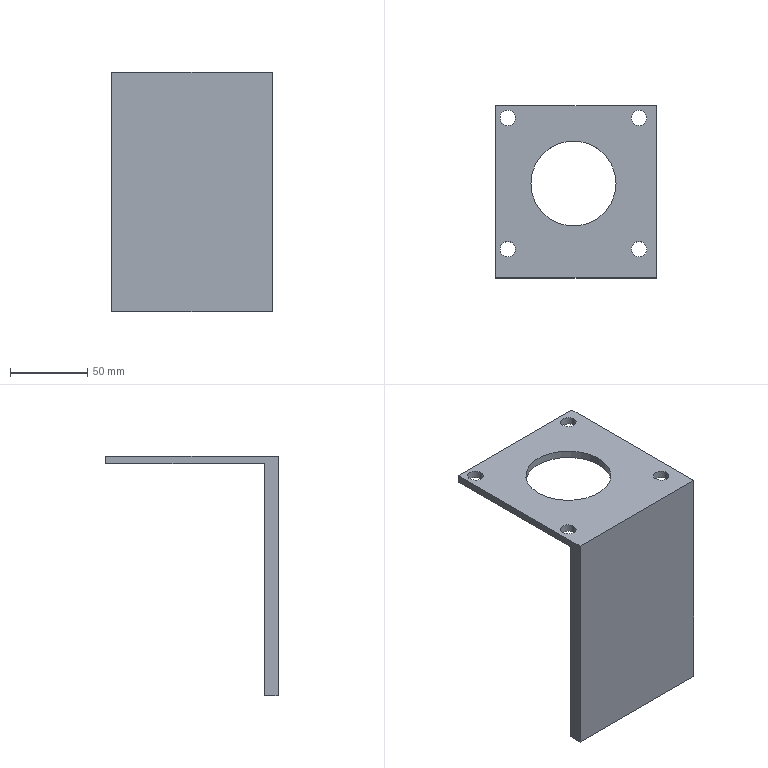Part | SolidWorks | features ICE 2, Cut 1, Extrusion 1 | 1 solid | 18 faces | box 104 x 111.35 x 155 mm | volume 184852 mm3 | cylinder 10 | plane 8 | commonest cylinder face diameters 10 x8 55 x2
STEP:
#1=CARTESIAN_POINT('',(47.426,-42.426,5.));
#2=VERTEX_POINT('',#1);
#3=CARTESIAN_POINT('',(37.426,-42.426,5.));
#4=VERTEX_POINT('',#3);
#5=CARTESIAN_POINT('',(42.426,-42.426,5.));
#6=DIRECTION('',(0.,0.,-1.));
#7=DIRECTION('',(-1.,0.,0.));
#8=AXIS2_PLACEMENT_3D('',#5,#6,#7);
#9=CIRCLE('',#8,5.);
#10=EDGE_CURVE('',#2,#4,#9,.T.);
#11=ORIENTED_EDGE('',*,*,#10,.F.);
#12=CARTESIAN_POINT('',(47.426,-42.426,0.));
#13=VERTEX_POINT('',#12);
#14=CARTESIAN_POINT('',(47.426,-42.426,5.));
#15=DIRECTION('',(0.,0.,-1.));
#16=VECTOR('',#15,1000.);
#17=LINE('',#14,#16);
#18=EDGE_CURVE('',#2,#13,#17,.T.);
#19=ORIENTED_EDGE('',*,*,#18,.T.);
#20=CARTESIAN_POINT('',(37.426,-42.426,0.));
#21=VERTEX_POINT('',#20);
#22=CARTESIAN_POINT('',(42.426,-42.426,0.));
#23=DIRECTION('',(0.,0.,-1.));
#24=DIRECTION('',(-1.,0.,0.));
#25=AXIS2_PLACEMENT_3D('',#22,#23,#24);
#26=CIRCLE('',#25,5.);
#27=EDGE_CURVE('',#13,#21,#26,.T.);
#28=ORIENTED_EDGE('',*,*,#27,.T.);
#29=CARTESIAN_POINT('',(37.426,-42.426,5.));
#30=DIRECTION('',(0.,0.,-1.));
#31=VECTOR('',#30,1000.);
#32=LINE('',#29,#31);
#33=EDGE_CURVE('',#4,#21,#32,.T.);
#34=ORIENTED_EDGE('',*,*,#33,.F.);
#35=EDGE_LOOP('',(#11,#19,#28,#34));
#36=FACE_OUTER_BOUND('',#35,.T.);
#37=CARTESIAN_POINT('',(42.426,-42.426,5.));
#38=DIRECTION('',(0.,0.,-1.));
#39=DIRECTION('',(-1.,0.,0.));
#40=AXIS2_PLACEMENT_3D('',#37,#38,#39);
#41=CYLINDRICAL_SURFACE('',#40,5.);
#42=ADVANCED_FACE('',(#36),#41,.F.);
#43=CARTESIAN_POINT('',(-37.426,-42.426,5.));
#44=VERTEX_POINT('',#43);
#45=CARTESIAN_POINT('',(-47.426,-42.426,5.));
#46=VERTEX_POINT('',#45);
#47=CARTESIAN_POINT('',(-42.426,-42.426,5.));
#48=DIRECTION('',(0.,0.,-1.));
#49=DIRECTION('',(-1.,0.,0.));
#50=AXIS2_PLACEMENT_3D('',#47,#48,#49);
#51=CIRCLE('',#50,5.);
#52=EDGE_CURVE('',#44,#46,#51,.T.);
#53=ORIENTED_EDGE('',*,*,#52,.F.);
#54=CARTESIAN_POINT('',(-37.426,-42.426,0.));
#55=VERTEX_POINT('',#54);
#56=CARTESIAN_POINT('',(-37.426,-42.426,5.));
#57=DIRECTION('',(0.,0.,-1.));
#58=VECTOR('',#57,1000.);
#59=LINE('',#56,#58);
#60=EDGE_CURVE('',#44,#55,#59,.T.);
#61=ORIENTED_EDGE('',*,*,#60,.T.);
#62=CARTESIAN_POINT('',(-47.426,-42.426,0.));
#63=VERTEX_POINT('',#62);
#64=CARTESIAN_POINT('',(-42.426,-42.426,0.));
#65=DIRECTION('',(0.,0.,-1.));
#66=DIRECTION('',(-1.,0.,0.));
#67=AXIS2_PLACEMENT_3D('',#64,#65,#66);
#68=CIRCLE('',#67,5.);
#69=EDGE_CURVE('',#55,#63,#68,.T.);
#70=ORIENTED_EDGE('',*,*,#69,.T.);
#71=CARTESIAN_POINT('',(-47.426,-42.426,5.));
#72=DIRECTION('',(0.,0.,-1.));
#73=VECTOR('',#72,1000.);
#74=LINE('',#71,#73);
#75=EDGE_CURVE('',#46,#63,#74,.T.);
#76=ORIENTED_EDGE('',*,*,#75,.F.);
#77=EDGE_LOOP('',(#53,#61,#70,#76));
#78=FACE_OUTER_BOUND('',#77,.T.);
#79=CARTESIAN_POINT('',(-42.426,-42.426,5.));
#80=DIRECTION('',(0.,0.,-1.));
#81=DIRECTION('',(-1.,0.,0.));
#82=AXIS2_PLACEMENT_3D('',#79,#80,#81);
#83=CYLINDRICAL_SURFACE('',#82,5.);
#84=ADVANCED_FACE('',(#78),#83,.F.);
#85=CARTESIAN_POINT('',(-37.426,42.426,5.));
#86=VERTEX_POINT('',#85);
#87=CARTESIAN_POINT('',(-47.426,42.426,5.));
#88=VERTEX_POINT('',#87);
#89=CARTESIAN_POINT('',(-42.426,42.426,5.));
#90=DIRECTION('',(0.,0.,-1.));
#91=DIRECTION('',(-1.,0.,0.));
#92=AXIS2_PLACEMENT_3D('',#89,#90,#91);
#93=CIRCLE('',#92,5.);
#94=EDGE_CURVE('',#86,#88,#93,.T.);
#95=ORIENTED_EDGE('',*,*,#94,.F.);
#96=CARTESIAN_POINT('',(-37.426,42.426,0.));
#97=VERTEX_POINT('',#96);
#98=CARTESIAN_POINT('',(-37.426,42.426,5.));
#99=DIRECTION('',(0.,0.,-1.));
#100=VECTOR('',#99,1000.);
#101=LINE('',#98,#100);
#102=EDGE_CURVE('',#86,#97,#101,.T.);
#103=ORIENTED_EDGE('',*,*,#102,.T.);
#104=CARTESIAN_POINT('',(-47.426,42.426,0.));
#105=VERTEX_POINT('',#104);
#106=CARTESIAN_POINT('',(-42.426,42.426,0.));
#107=DIRECTION('',(0.,0.,-1.));
#108=DIRECTION('',(-1.,0.,0.));
#109=AXIS2_PLACEMENT_3D('',#106,#107,#108);
#110=CIRCLE('',#109,5.);
#111=EDGE_CURVE('',#97,#105,#110,.T.);
#112=ORIENTED_EDGE('',*,*,#111,.T.);
#113=CARTESIAN_POINT('',(-47.426,42.426,5.));
#114=DIRECTION('',(0.,0.,-1.));
#115=VECTOR('',#114,1000.);
#116=LINE('',#113,#115);
#117=EDGE_CURVE('',#88,#105,#116,.T.);
#118=ORIENTED_EDGE('',*,*,#117,.F.);
#119=EDGE_LOOP('',(#95,#103,#112,#118));
#120=FACE_OUTER_BOUND('',#119,.T.);
#121=CARTESIAN_POINT('',(-42.426,42.426,5.));
#122=DIRECTION('',(0.,0.,-1.));
#123=DIRECTION('',(-1.,0.,0.));
#124=AXIS2_PLACEMENT_3D('',#121,#122,#123);
#125=CYLINDRICAL_SURFACE('',#124,5.);
#126=ADVANCED_FACE('',(#120),#125,.F.);
#127=CARTESIAN_POINT('',(47.426,42.426,5.));
#128=VERTEX_POINT('',#127);
#129=CARTESIAN_POINT('',(37.426,42.426,5.));
#130=VERTEX_POINT('',#129);
#131=CARTESIAN_POINT('',(42.426,42.426,5.));
#132=DIRECTION('',(0.,0.,-1.));
#133=DIRECTION('',(-1.,0.,0.));
#134=AXIS2_PLACEMENT_3D('',#131,#132,#133);
#135=CIRCLE('',#134,5.);
#136=EDGE_CURVE('',#128,#130,#135,.T.);
#137=ORIENTED_EDGE('',*,*,#136,.F.);
#138=CARTESIAN_POINT('',(47.426,42.426,0.));
#139=VERTEX_POINT('',#138);
#140=CARTESIAN_POINT('',(47.426,42.426,5.));
#141=DIRECTION('',(0.,0.,-1.));
#142=VECTOR('',#141,1000.);
#143=LINE('',#140,#142);
#144=EDGE_CURVE('',#128,#139,#143,.T.);
#145=ORIENTED_EDGE('',*,*,#144,.T.);
#146=CARTESIAN_POINT('',(37.426,42.426,0.));
#147=VERTEX_POINT('',#146);
#148=CARTESIAN_POINT('',(42.426,42.426,0.));
#149=DIRECTION('',(0.,0.,-1.));
#150=DIRECTION('',(-1.,0.,0.));
#151=AXIS2_PLACEMENT_3D('',#148,#149,#150);
#152=CIRCLE('',#151,5.);
#153=EDGE_CURVE('',#139,#147,#152,.T.);
#154=ORIENTED_EDGE('',*,*,#153,.T.);
#155=CARTESIAN_POINT('',(37.426,42.426,5.));
#156=DIRECTION('',(0.,0.,-1.));
#157=VECTOR('',#156,1000.);
#158=LINE('',#155,#157);
#159=EDGE_CURVE('',#130,#147,#158,.T.);
#160=ORIENTED_EDGE('',*,*,#159,.F.);
#161=EDGE_LOOP('',(#137,#145,#154,#160));
#162=FACE_OUTER_BOUND('',#161,.T.);
#163=CARTESIAN_POINT('',(42.426,42.426,5.));
#164=DIRECTION('',(0.,0.,-1.));
#165=DIRECTION('',(-1.,0.,0.));
#166=AXIS2_PLACEMENT_3D('',#163,#164,#165);
#167=CYLINDRICAL_SURFACE('',#166,5.);
#168=ADVANCED_FACE('',(#162),#167,.F.);
#169=CARTESIAN_POINT('',(27.5,0.,0.));
#170=VERTEX_POINT('',#169);
#171=CARTESIAN_POINT('',(-27.5,0.,0.));
#172=VERTEX_POINT('',#171);
#173=CARTESIAN_POINT('',(0.,0.,0.));
#174=DIRECTION('',(0.,0.,-1.));
#175=DIRECTION('',(-1.,0.,0.));
#176=AXIS2_PLACEMENT_3D('',#173,#174,#175);
#177=CIRCLE('',#176,27.5);
#178=EDGE_CURVE('',#170,#172,#177,.T.);
#179=ORIENTED_EDGE('',*,*,#178,.T.);
#180=CARTESIAN_POINT('',(-27.5,0.,5.));
#181=VERTEX_POINT('',#180);
#182=CARTESIAN_POINT('',(-27.5,0.,-15.));
#183=DIRECTION('',(0.,0.,1.));
#184=VECTOR('',#183,1000.);
#185=LINE('',#182,#184);
#186=EDGE_CURVE('',#172,#181,#185,.T.);
#187=ORIENTED_EDGE('',*,*,#186,.T.);
#188=CARTESIAN_POINT('',(27.5,0.,5.));
#189=VERTEX_POINT('',#188);
#190=CARTESIAN_POINT('',(0.,0.,5.));
#191=DIRECTION('',(0.,0.,1.));
#192=DIRECTION('',(1.,0.,0.));
#193=AXIS2_PLACEMENT_3D('',#190,#191,#192);
#194=CIRCLE('',#193,27.5);
#195=EDGE_CURVE('',#181,#189,#194,.T.);
#196=ORIENTED_EDGE('',*,*,#195,.T.);
#197=CARTESIAN_POINT('',(27.5,0.,-15.));
#198=DIRECTION('',(0.,0.,1.));
#199=VECTOR('',#198,1000.);
#200=LINE('',#197,#199);
#201=EDGE_CURVE('',#170,#189,#200,.T.);
#202=ORIENTED_EDGE('',*,*,#201,.F.);
#203=EDGE_LOOP('',(#179,#187,#196,#202));
#204=FACE_OUTER_BOUND('',#203,.T.);
#205=CARTESIAN_POINT('',(0.,0.,-15.));
#206=DIRECTION('',(0.,0.,1.));
#207=DIRECTION('',(1.,0.,0.));
#208=AXIS2_PLACEMENT_3D('',#205,#206,#207);
#209=CYLINDRICAL_SURFACE('',#208,27.5);
#210=ADVANCED_FACE('',(#204),#209,.F.);
#211=CARTESIAN_POINT('',(53.645,50.355,0.));
#212=VERTEX_POINT('',#211);
#213=CARTESIAN_POINT('',(-50.355,50.355,0.));
#214=VERTEX_POINT('',#213);
#215=CARTESIAN_POINT('',(-50.355,50.355,0.));
#216=DIRECTION('',(-1.,0.,0.));
#217=VECTOR('',#216,1000.);
#218=LINE('',#215,#217);
#219=EDGE_CURVE('',#212,#214,#218,.T.);
#220=ORIENTED_EDGE('',*,*,#219,.T.);
#221=CARTESIAN_POINT('',(-50.355,50.355,5.));
#222=VERTEX_POINT('',#221);
#223=CARTESIAN_POINT('',(-50.355,50.355,5.));
#224=DIRECTION('',(0.,0.,-1.));
#225=VECTOR('',#224,1000.);
#226=LINE('',#223,#225);
#227=EDGE_CURVE('',#222,#214,#226,.T.);
#228=ORIENTED_EDGE('',*,*,#227,.F.);
#229=CARTESIAN_POINT('',(53.645,50.355,5.));
#230=VERTEX_POINT('',#229);
#231=CARTESIAN_POINT('',(-50.355,50.355,5.));
#232=DIRECTION('',(-1.,0.,0.));
#233=VECTOR('',#232,1000.);
#234=LINE('',#231,#233);
#235=EDGE_CURVE('',#230,#222,#234,.T.);
#236=ORIENTED_EDGE('',*,*,#235,.F.);
#237=CARTESIAN_POINT('',(53.645,50.355,5.));
#238=DIRECTION('',(0.,0.,-1.));
#239=VECTOR('',#238,1000.);
#240=LINE('',#237,#239);
#241=EDGE_CURVE('',#230,#212,#240,.T.);
#242=ORIENTED_EDGE('',*,*,#241,.T.);
#243=EDGE_LOOP('',(#220,#228,#236,#242));
#244=FACE_OUTER_BOUND('',#243,.T.);
#245=CARTESIAN_POINT('',(-50.355,50.355,5.));
#246=DIRECTION('',(0.,-1.,0.));
#247=DIRECTION('',(0.,0.,-1.));
#248=AXIS2_PLACEMENT_3D('',#245,#246,#247);
#249=PLANE('',#248);
#250=ADVANCED_FACE('',(#244),#249,.F.);
#251=CARTESIAN_POINT('',(-50.355,-51.995,0.));
#252=VERTEX_POINT('',#251);
#253=CARTESIAN_POINT('',(-50.355,-53.645,0.));
#254=DIRECTION('',(0.,-1.,0.));
#255=VECTOR('',#254,1000.);
#256=LINE('',#253,#255);
#257=EDGE_CURVE('',#214,#252,#256,.T.);
#258=ORIENTED_EDGE('',*,*,#257,.T.);
#259=CARTESIAN_POINT('',(-50.355,-51.995,-150.));
#260=VERTEX_POINT('',#259);
#261=CARTESIAN_POINT('',(-50.355,-51.995,-150.));
#262=DIRECTION('',(0.,0.,1.));
#263=VECTOR('',#262,1000.);
#264=LINE('',#261,#263);
#265=EDGE_CURVE('',#260,#252,#264,.T.);
#266=ORIENTED_EDGE('',*,*,#265,.F.);
#267=CARTESIAN_POINT('',(-50.355,-60.995,-150.));
#268=VERTEX_POINT('',#267);
#269=CARTESIAN_POINT('',(-50.355,-60.995,-150.));
#270=DIRECTION('',(0.,1.,0.));
#271=VECTOR('',#270,1000.);
#272=LINE('',#269,#271);
#273=EDGE_CURVE('',#268,#260,#272,.T.);
#274=ORIENTED_EDGE('',*,*,#273,.F.);
#275=CARTESIAN_POINT('',(-50.355,-60.995,5.));
#276=VERTEX_POINT('',#275);
#277=CARTESIAN_POINT('',(-50.355,-60.995,5.));
#278=DIRECTION('',(0.,0.,-1.));
#279=VECTOR('',#278,1000.);
#280=LINE('',#277,#279);
#281=EDGE_CURVE('',#276,#268,#280,.T.);
#282=ORIENTED_EDGE('',*,*,#281,.F.);
#283=CARTESIAN_POINT('',(-50.355,-47.266,5.));
#284=DIRECTION('',(0.,-1.,0.));
#285=VECTOR('',#284,1000.);
#286=LINE('',#283,#285);
#287=EDGE_CURVE('',#222,#276,#286,.T.);
#288=ORIENTED_EDGE('',*,*,#287,.F.);
#289=ORIENTED_EDGE('',*,*,#227,.T.);
#290=EDGE_LOOP('',(#258,#266,#274,#282,#288,#289));
#291=FACE_OUTER_BOUND('',#290,.T.);
#292=CARTESIAN_POINT('',(-50.355,-53.645,5.));
#293=DIRECTION('',(1.,0.,0.));
#294=DIRECTION('',(0.,0.,-1.));
#295=AXIS2_PLACEMENT_3D('',#292,#293,#294);
#296=PLANE('',#295);
#297=ADVANCED_FACE('',(#291),#296,.F.);
#298=ORIENTED_EDGE('',*,*,#281,.T.);
#299=CARTESIAN_POINT('',(53.645,-60.995,-150.));
#300=VERTEX_POINT('',#299);
#301=CARTESIAN_POINT('',(53.645,-60.995,-150.));
#302=DIRECTION('',(-1.,0.,0.));
#303=VECTOR('',#302,1000.);
#304=LINE('',#301,#303);
#305=EDGE_CURVE('',#300,#268,#304,.T.);
#306=ORIENTED_EDGE('',*,*,#305,.F.);
#307=CARTESIAN_POINT('',(53.645,-60.995,5.));
#308=VERTEX_POINT('',#307);
#309=CARTESIAN_POINT('',(53.645,-60.995,5.));
#310=DIRECTION('',(0.,0.,-1.));
#311=VECTOR('',#310,1000.);
#312=LINE('',#309,#311);
#313=EDGE_CURVE('',#308,#300,#312,.T.);
#314=ORIENTED_EDGE('',*,*,#313,.F.);
#315=CARTESIAN_POINT('',(-50.355,-60.995,5.));
#316=DIRECTION('',(1.,0.,0.));
#317=VECTOR('',#316,1000.);
#318=LINE('',#315,#317);
#319=EDGE_CURVE('',#276,#308,#318,.T.);
#320=ORIENTED_EDGE('',*,*,#319,.F.);
#321=EDGE_LOOP('',(#298,#306,#314,#320));
#322=FACE_OUTER_BOUND('',#321,.T.);
#323=CARTESIAN_POINT('',(-50.355,-60.995,5.));
#324=DIRECTION('',(0.,1.,0.));
#325=DIRECTION('',(0.,0.,1.));
#326=AXIS2_PLACEMENT_3D('',#323,#324,#325);
#327=PLANE('',#326);
#328=ADVANCED_FACE('',(#322),#327,.F.);
#329=ORIENTED_EDGE('',*,*,#313,.T.);
#330=CARTESIAN_POINT('',(53.645,-51.995,-150.));
#331=VERTEX_POINT('',#330);
#332=CARTESIAN_POINT('',(53.645,-60.995,-150.));
#333=DIRECTION('',(0.,-1.,0.));
#334=VECTOR('',#333,1000.);
#335=LINE('',#332,#334);
#336=EDGE_CURVE('',#331,#300,#335,.T.);
#337=ORIENTED_EDGE('',*,*,#336,.F.);
#338=CARTESIAN_POINT('',(53.645,-51.995,0.));
#339=VERTEX_POINT('',#338);
#340=CARTESIAN_POINT('',(53.645,-51.995,-150.));
#341=DIRECTION('',(0.,0.,1.));
#342=VECTOR('',#341,1000.);
#343=LINE('',#340,#342);
#344=EDGE_CURVE('',#331,#339,#343,.T.);
#345=ORIENTED_EDGE('',*,*,#344,.T.);
#346=CARTESIAN_POINT('',(53.645,-60.995,0.));
#347=DIRECTION('',(0.,1.,0.));
#348=VECTOR('',#347,1000.);
#349=LINE('',#346,#348);
#350=EDGE_CURVE('',#339,#212,#349,.T.);
#351=ORIENTED_EDGE('',*,*,#350,.T.);
#352=ORIENTED_EDGE('',*,*,#241,.F.);
#353=CARTESIAN_POINT('',(53.645,-53.645,5.));
#354=DIRECTION('',(0.,1.,0.));
#355=VECTOR('',#354,1000.);
#356=LINE('',#353,#355);
#357=EDGE_CURVE('',#308,#230,#356,.T.);
#358=ORIENTED_EDGE('',*,*,#357,.F.);
#359=EDGE_LOOP('',(#329,#337,#345,#351,#352,#358));
#360=FACE_OUTER_BOUND('',#359,.T.);
#361=CARTESIAN_POINT('',(53.645,-60.995,5.));
#362=DIRECTION('',(-1.,0.,0.));
#363=DIRECTION('',(0.,0.,1.));
#364=AXIS2_PLACEMENT_3D('',#361,#362,#363);
#365=PLANE('',#364);
#366=ADVANCED_FACE('',(#360),#365,.F.);
#367=CARTESIAN_POINT('',(42.426,-42.426,5.));
#368=DIRECTION('',(0.,0.,-1.));
#369=DIRECTION('',(-1.,0.,0.));
#370=AXIS2_PLACEMENT_3D('',#367,#368,#369);
#371=CIRCLE('',#370,5.);
#372=EDGE_CURVE('',#4,#2,#371,.T.);
#373=ORIENTED_EDGE('',*,*,#372,.T.);
#374=ORIENTED_EDGE('',*,*,#10,.T.);
#375=EDGE_LOOP('',(#373,#374));
#376=FACE_BOUND('',#375,.T.);
#377=CARTESIAN_POINT('',(-42.426,-42.426,5.));
#378=DIRECTION('',(0.,0.,-1.));
#379=DIRECTION('',(-1.,0.,0.));
#380=AXIS2_PLACEMENT_3D('',#377,#378,#379);
#381=CIRCLE('',#380,5.);
#382=EDGE_CURVE('',#46,#44,#381,.T.);
#383=ORIENTED_EDGE('',*,*,#382,.T.);
#384=ORIENTED_EDGE('',*,*,#52,.T.);
#385=EDGE_LOOP('',(#383,#384));
#386=FACE_BOUND('',#385,.T.);
#387=CARTESIAN_POINT('',(-42.426,42.426,5.));
#388=DIRECTION('',(0.,0.,-1.));
#389=DIRECTION('',(-1.,0.,0.));
#390=AXIS2_PLACEMENT_3D('',#387,#388,#389);
#391=CIRCLE('',#390,5.);
#392=EDGE_CURVE('',#88,#86,#391,.T.);
#393=ORIENTED_EDGE('',*,*,#392,.T.);
#394=ORIENTED_EDGE('',*,*,#94,.T.);
#395=EDGE_LOOP('',(#393,#394));
#396=FACE_BOUND('',#395,.T.);
#397=CARTESIAN_POINT('',(42.426,42.426,5.));
#398=DIRECTION('',(0.,0.,-1.));
#399=DIRECTION('',(-1.,0.,0.));
#400=AXIS2_PLACEMENT_3D('',#397,#398,#399);
#401=CIRCLE('',#400,5.);
#402=EDGE_CURVE('',#130,#128,#401,.T.);
#403=ORIENTED_EDGE('',*,*,#402,.T.);
#404=ORIENTED_EDGE('',*,*,#136,.T.);
#405=EDGE_LOOP('',(#403,#404));
#406=FACE_BOUND('',#405,.T.);
#407=CARTESIAN_POINT('',(0.,0.,5.));
#408=DIRECTION('',(0.,0.,1.));
#409=DIRECTION('',(1.,0.,0.));
#410=AXIS2_PLACEMENT_3D('',#407,#408,#409);
#411=CIRCLE('',#410,27.5);
#412=EDGE_CURVE('',#189,#181,#411,.T.);
#413=ORIENTED_EDGE('',*,*,#412,.F.);
#414=ORIENTED_EDGE('',*,*,#195,.F.);
#415=EDGE_LOOP('',(#413,#414));
#416=FACE_BOUND('',#415,.T.);
#417=ORIENTED_EDGE('',*,*,#357,.T.);
#418=ORIENTED_EDGE('',*,*,#235,.T.);
#419=ORIENTED_EDGE('',*,*,#287,.T.);
#420=ORIENTED_EDGE('',*,*,#319,.T.);
#421=EDGE_LOOP('',(#417,#418,#419,#420));
#422=FACE_OUTER_BOUND('',#421,.T.);
#423=CARTESIAN_POINT('',(0.,0.,5.));
#424=DIRECTION('',(0.,0.,-1.));
#425=DIRECTION('',(-1.,0.,0.));
#426=AXIS2_PLACEMENT_3D('',#423,#424,#425);
#427=PLANE('',#426);
#428=ADVANCED_FACE('',(#376,#386,#396,#406,#416,#422),#427,.F.);
#429=CARTESIAN_POINT('',(42.426,-42.426,0.));
#430=DIRECTION('',(0.,0.,-1.));
#431=DIRECTION('',(-1.,0.,0.));
#432=AXIS2_PLACEMENT_3D('',#429,#430,#431);
#433=CIRCLE('',#432,5.);
#434=EDGE_CURVE('',#21,#13,#433,.T.);
#435=ORIENTED_EDGE('',*,*,#434,.F.);
#436=ORIENTED_EDGE('',*,*,#27,.F.);
#437=EDGE_LOOP('',(#435,#436));
#438=FACE_BOUND('',#437,.T.);
#439=CARTESIAN_POINT('',(-42.426,-42.426,0.));
#440=DIRECTION('',(0.,0.,-1.));
#441=DIRECTION('',(-1.,0.,0.));
#442=AXIS2_PLACEMENT_3D('',#439,#440,#441);
#443=CIRCLE('',#442,5.);
#444=EDGE_CURVE('',#63,#55,#443,.T.);
#445=ORIENTED_EDGE('',*,*,#444,.F.);
#446=ORIENTED_EDGE('',*,*,#69,.F.);
#447=EDGE_LOOP('',(#445,#446));
#448=FACE_BOUND('',#447,.T.);
#449=CARTESIAN_POINT('',(-42.426,42.426,0.));
#450=DIRECTION('',(0.,0.,-1.));
#451=DIRECTION('',(-1.,0.,0.));
#452=AXIS2_PLACEMENT_3D('',#449,#450,#451);
#453=CIRCLE('',#452,5.);
#454=EDGE_CURVE('',#105,#97,#453,.T.);
#455=ORIENTED_EDGE('',*,*,#454,.F.);
#456=ORIENTED_EDGE('',*,*,#111,.F.);
#457=EDGE_LOOP('',(#455,#456));
#458=FACE_BOUND('',#457,.T.);
#459=CARTESIAN_POINT('',(42.426,42.426,0.));
#460=DIRECTION('',(0.,0.,-1.));
#461=DIRECTION('',(-1.,0.,0.));
#462=AXIS2_PLACEMENT_3D('',#459,#460,#461);
#463=CIRCLE('',#462,5.);
#464=EDGE_CURVE('',#147,#139,#463,.T.);
#465=ORIENTED_EDGE('',*,*,#464,.F.);
#466=ORIENTED_EDGE('',*,*,#153,.F.);
#467=EDGE_LOOP('',(#465,#466));
#468=FACE_BOUND('',#467,.T.);
#469=CARTESIAN_POINT('',(53.645,-51.995,0.));
#470=DIRECTION('',(1.,0.,0.));
#471=VECTOR('',#470,1000.);
#472=LINE('',#469,#471);
#473=EDGE_CURVE('',#252,#339,#472,.T.);
#474=ORIENTED_EDGE('',*,*,#473,.F.);
#475=ORIENTED_EDGE('',*,*,#257,.F.);
#476=ORIENTED_EDGE('',*,*,#219,.F.);
#477=ORIENTED_EDGE('',*,*,#350,.F.);
#478=EDGE_LOOP('',(#474,#475,#476,#477));
#479=FACE_OUTER_BOUND('',#478,.T.);
#480=ORIENTED_EDGE('',*,*,#178,.F.);
#481=CARTESIAN_POINT('',(0.,0.,0.));
#482=DIRECTION('',(0.,0.,-1.));
#483=DIRECTION('',(-1.,0.,0.));
#484=AXIS2_PLACEMENT_3D('',#481,#482,#483);
#485=CIRCLE('',#484,27.5);
#486=EDGE_CURVE('',#172,#170,#485,.T.);
#487=ORIENTED_EDGE('',*,*,#486,.F.);
#488=EDGE_LOOP('',(#480,#487));
#489=FACE_BOUND('',#488,.T.);
#490=CARTESIAN_POINT('',(0.,0.,0.));
#491=DIRECTION('',(0.,0.,-1.));
#492=DIRECTION('',(-1.,0.,0.));
#493=AXIS2_PLACEMENT_3D('',#490,#491,#492);
#494=PLANE('',#493);
#495=ADVANCED_FACE('',(#438,#448,#458,#468,#479,#489),#494,.T.);
#496=ORIENTED_EDGE('',*,*,#186,.F.);
#497=ORIENTED_EDGE('',*,*,#486,.T.);
#498=ORIENTED_EDGE('',*,*,#201,.T.);
#499=ORIENTED_EDGE('',*,*,#412,.T.);
#500=EDGE_LOOP('',(#496,#497,#498,#499));
#501=FACE_OUTER_BOUND('',#500,.T.);
#502=CARTESIAN_POINT('',(0.,0.,-15.));
#503=DIRECTION('',(0.,0.,1.));
#504=DIRECTION('',(1.,0.,0.));
#505=AXIS2_PLACEMENT_3D('',#502,#503,#504);
#506=CYLINDRICAL_SURFACE('',#505,27.5);
#507=ADVANCED_FACE('',(#501),#506,.F.);
#508=ORIENTED_EDGE('',*,*,#473,.T.);
#509=ORIENTED_EDGE('',*,*,#344,.F.);
#510=CARTESIAN_POINT('',(53.645,-51.995,-150.));
#511=DIRECTION('',(1.,0.,0.));
#512=VECTOR('',#511,1000.);
#513=LINE('',#510,#512);
#514=EDGE_CURVE('',#260,#331,#513,.T.);
#515=ORIENTED_EDGE('',*,*,#514,.F.);
#516=ORIENTED_EDGE('',*,*,#265,.T.);
#517=EDGE_LOOP('',(#508,#509,#515,#516));
#518=FACE_OUTER_BOUND('',#517,.T.);
#519=CARTESIAN_POINT('',(53.645,-51.995,-150.));
#520=DIRECTION('',(0.,-1.,0.));
#521=DIRECTION('',(0.,0.,-1.));
#522=AXIS2_PLACEMENT_3D('',#519,#520,#521);
#523=PLANE('',#522);
#524=ADVANCED_FACE('',(#518),#523,.F.);
#525=ORIENTED_EDGE('',*,*,#336,.T.);
#526=ORIENTED_EDGE('',*,*,#305,.T.);
#527=ORIENTED_EDGE('',*,*,#273,.T.);
#528=ORIENTED_EDGE('',*,*,#514,.T.);
#529=EDGE_LOOP('',(#525,#526,#527,#528));
#530=FACE_OUTER_BOUND('',#529,.T.);
#531=CARTESIAN_POINT('',(0.,0.,-150.));
#532=DIRECTION('',(0.,0.,1.));
#533=DIRECTION('',(1.,0.,0.));
#534=AXIS2_PLACEMENT_3D('',#531,#532,#533);
#535=PLANE('',#534);
#536=ADVANCED_FACE('',(#530),#535,.F.);
#537=ORIENTED_EDGE('',*,*,#144,.F.);
#538=ORIENTED_EDGE('',*,*,#402,.F.);
#539=ORIENTED_EDGE('',*,*,#159,.T.);
#540=ORIENTED_EDGE('',*,*,#464,.T.);
#541=EDGE_LOOP('',(#537,#538,#539,#540));
#542=FACE_OUTER_BOUND('',#541,.T.);
#543=CARTESIAN_POINT('',(42.426,42.426,5.));
#544=DIRECTION('',(0.,0.,-1.));
#545=DIRECTION('',(-1.,0.,0.));
#546=AXIS2_PLACEMENT_3D('',#543,#544,#545);
#547=CYLINDRICAL_SURFACE('',#546,5.);
#548=ADVANCED_FACE('',(#542),#547,.F.);
#549=ORIENTED_EDGE('',*,*,#102,.F.);
#550=ORIENTED_EDGE('',*,*,#392,.F.);
#551=ORIENTED_EDGE('',*,*,#117,.T.);
#552=ORIENTED_EDGE('',*,*,#454,.T.);
#553=EDGE_LOOP('',(#549,#550,#551,#552));
#554=FACE_OUTER_BOUND('',#553,.T.);
#555=CARTESIAN_POINT('',(-42.426,42.426,5.));
#556=DIRECTION('',(0.,0.,-1.));
#557=DIRECTION('',(-1.,0.,0.));
#558=AXIS2_PLACEMENT_3D('',#555,#556,#557);
#559=CYLINDRICAL_SURFACE('',#558,5.);
#560=ADVANCED_FACE('',(#554),#559,.F.);
#561=ORIENTED_EDGE('',*,*,#60,.F.);
#562=ORIENTED_EDGE('',*,*,#382,.F.);
#563=ORIENTED_EDGE('',*,*,#75,.T.);
#564=ORIENTED_EDGE('',*,*,#444,.T.);
#565=EDGE_LOOP('',(#561,#562,#563,#564));
#566=FACE_OUTER_BOUND('',#565,.T.);
#567=CARTESIAN_POINT('',(-42.426,-42.426,5.));
#568=DIRECTION('',(0.,0.,-1.));
#569=DIRECTION('',(-1.,0.,0.));
#570=AXIS2_PLACEMENT_3D('',#567,#568,#569);
#571=CYLINDRICAL_SURFACE('',#570,5.);
#572=ADVANCED_FACE('',(#566),#571,.F.);
#573=ORIENTED_EDGE('',*,*,#18,.F.);
#574=ORIENTED_EDGE('',*,*,#372,.F.);
#575=ORIENTED_EDGE('',*,*,#33,.T.);
#576=ORIENTED_EDGE('',*,*,#434,.T.);
#577=EDGE_LOOP('',(#573,#574,#575,#576));
#578=FACE_OUTER_BOUND('',#577,.T.);
#579=CARTESIAN_POINT('',(42.426,-42.426,5.));
#580=DIRECTION('',(0.,0.,-1.));
#581=DIRECTION('',(-1.,0.,0.));
#582=AXIS2_PLACEMENT_3D('',#579,#580,#581);
#583=CYLINDRICAL_SURFACE('',#582,5.);
#584=ADVANCED_FACE('',(#578),#583,.F.);
#585=CLOSED_SHELL('',(#42,#84,#126,#168,#210,#250,#297,#328,#366,#428,#495,#507,#524,#536,#548,#560,#572,#584));
#586=MANIFOLD_SOLID_BREP('',#585);
#587=CARTESIAN_POINT('',(0.,0.,0.));
#588=DIRECTION('',(0.,0.,1.));
#589=DIRECTION('',(1.,0.,0.));
#590=AXIS2_PLACEMENT_3D('',#587,#588,#589);
#591=(LENGTH_UNIT()NAMED_UNIT(*)SI_UNIT(.MILLI.,.METRE.));
#592=UNCERTAINTY_MEASURE_WITH_UNIT(LENGTH_MEASURE(0.00001),#591,'','');
#593=(NAMED_UNIT(*)PLANE_ANGLE_UNIT()SI_UNIT($,.RADIAN.));
#594=(NAMED_UNIT(*)SI_UNIT($,.STERADIAN.)SOLID_ANGLE_UNIT());
#595=(GEOMETRIC_REPRESENTATION_CONTEXT(3)GLOBAL_UNCERTAINTY_ASSIGNED_CONTEXT((#592))GLOBAL_UNIT_ASSIGNED_CONTEXT((#591,#593,#594))REPRESENTATION_CONTEXT('',''));
#596=ADVANCED_BREP_SHAPE_REPRESENTATION('',(#586,#590),#595);